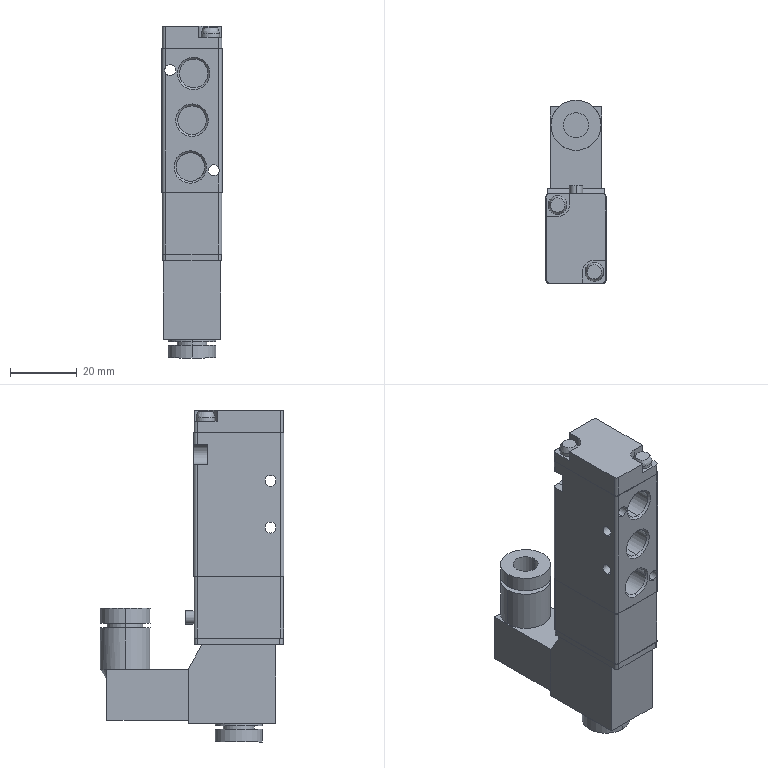Part | 1 solid | 132 faces | box 18 x 55 x 99.9 mm | volume 49289 mm3 | cylinder 60 | plane 59 | cone 11 | spline 2 | commonest cylinder face diameters 2 x18 8.566 x10 3.3 x8 5.6 x4 14.2 x4 15 x4